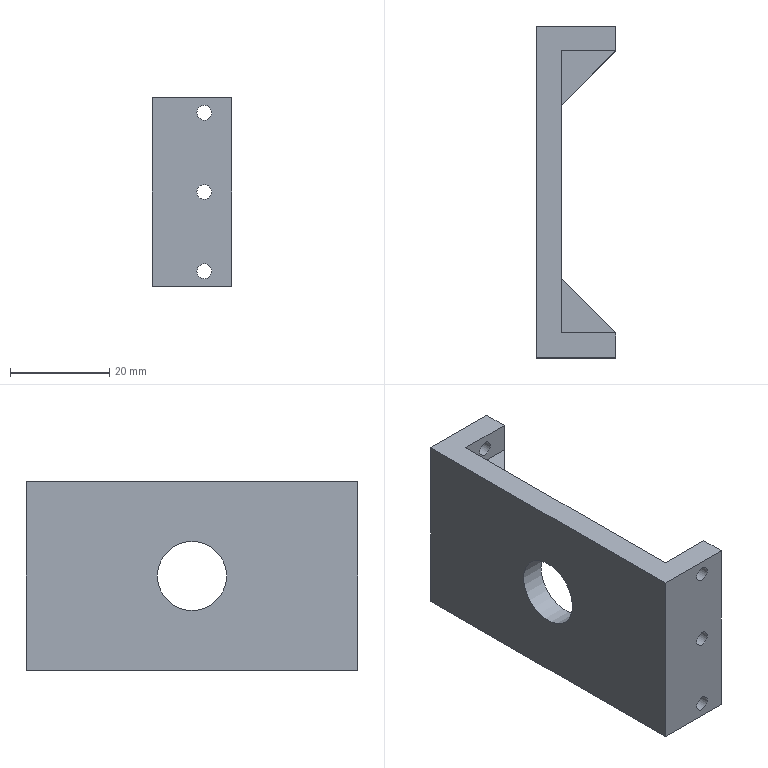Part | STEP file | 1-01.6 | 1 solid | 33 faces | box 16 x 67 x 38 mm | volume 16896 mm3 | plane 26 | cylinder 7 | commonest cylinder face diameters 3 x6 14 x1